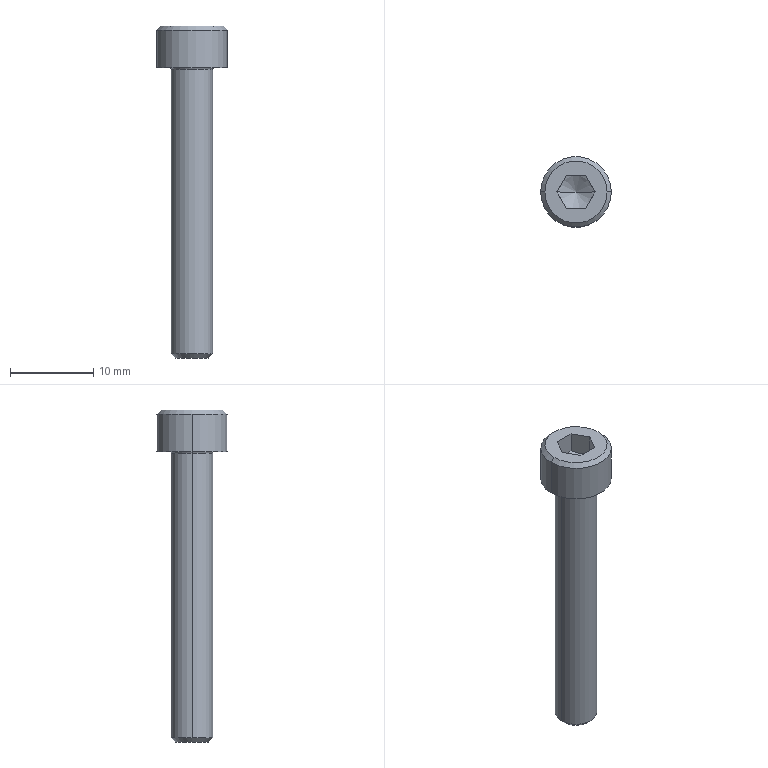Part | Creo | 1 solid | 23 faces | box 8.5 x 8.5 x 40 mm | volume 924.163 mm3 | plane 9 | cone 6 | cylinder 4 | torus 4 | commonest cylinder face diameters 5 x2 8.5 x2
STEP:
#1=CARTESIAN_POINT('',(0.,0.,0.));
#2=DIRECTION('',(0.,0.,1.));
#3=DIRECTION('',(1.,0.,0.));
#4=AXIS2_PLACEMENT_3D('',#1,#2,#3);
#5=CARTESIAN_POINT('',(-132.691,152.,16.));
#6=VERTEX_POINT('',#5);
#7=CARTESIAN_POINT('',(-133.845,154.,16.));
#8=VERTEX_POINT('',#7);
#9=CARTESIAN_POINT('',(-132.691,152.,16.));
#10=CARTESIAN_POINT('',(-132.753,152.109,15.964));
#11=CARTESIAN_POINT('',(-132.88,152.327,15.9));
#12=CARTESIAN_POINT('',(-133.073,152.663,15.836));
#13=CARTESIAN_POINT('',(-133.268,153.001,15.814));
#14=CARTESIAN_POINT('',(-133.464,153.339,15.836));
#15=CARTESIAN_POINT('',(-133.657,153.674,15.9));
#16=CARTESIAN_POINT('',(-133.783,153.892,15.964));
#17=CARTESIAN_POINT('',(-133.845,154.,16.));
#18=B_SPLINE_CURVE_WITH_KNOTS('',3,(#9,#10,#11,#12,#13,#14,#15,#16,#17),.UNSPECIFIED.,.F.,.F.,(4,1,1,1,1,1,4),(0.,0.1667,0.3333,0.5,0.6667,0.8333,1.),.UNSPECIFIED.);
#19=EDGE_CURVE('',#6,#8,#18,.T.);
#20=ORIENTED_EDGE('',*,*,#19,.F.);
#21=CARTESIAN_POINT('',(-135.,152.,14.667));
#22=VERTEX_POINT('',#21);
#23=CARTESIAN_POINT('',(-135.,152.,14.667));
#24=DIRECTION('',(0.866,0.,0.5));
#25=VECTOR('',#24,2.667);
#26=LINE('',#23,#25);
#27=EDGE_CURVE('',#22,#6,#26,.T.);
#28=ORIENTED_EDGE('',*,*,#27,.F.);
#29=CARTESIAN_POINT('',(-137.309,152.,16.));
#30=VERTEX_POINT('',#29);
#31=CARTESIAN_POINT('',(-135.,152.,14.667));
#32=DIRECTION('',(-0.866,0.,0.5));
#33=VECTOR('',#32,2.667);
#34=LINE('',#31,#33);
#35=EDGE_CURVE('',#22,#30,#34,.T.);
#36=ORIENTED_EDGE('',*,*,#35,.T.);
#37=CARTESIAN_POINT('',(-136.155,154.,16.));
#38=VERTEX_POINT('',#37);
#39=CARTESIAN_POINT('',(-136.155,154.,16.));
#40=CARTESIAN_POINT('',(-136.218,153.891,15.964));
#41=CARTESIAN_POINT('',(-136.344,153.673,15.9));
#42=CARTESIAN_POINT('',(-136.537,153.337,15.836));
#43=CARTESIAN_POINT('',(-136.733,152.999,15.814));
#44=CARTESIAN_POINT('',(-136.928,152.661,15.836));
#45=CARTESIAN_POINT('',(-137.121,152.326,15.9));
#46=CARTESIAN_POINT('',(-137.247,152.108,15.964));
#47=CARTESIAN_POINT('',(-137.309,152.,16.));
#48=B_SPLINE_CURVE_WITH_KNOTS('',3,(#39,#40,#41,#42,#43,#44,#45,#46,#47),.UNSPECIFIED.,.F.,.F.,(4,1,1,1,1,1,4),(0.,0.1667,0.3333,0.5,0.6667,0.8333,1.),.UNSPECIFIED.);
#49=EDGE_CURVE('',#38,#30,#48,.T.);
#50=ORIENTED_EDGE('',*,*,#49,.F.);
#51=CARTESIAN_POINT('',(-133.845,154.,16.));
#52=CARTESIAN_POINT('',(-133.919,154.,15.979));
#53=CARTESIAN_POINT('',(-134.064,154.,15.94));
#54=CARTESIAN_POINT('',(-134.273,154.,15.894));
#55=CARTESIAN_POINT('',(-134.479,154.,15.858));
#56=CARTESIAN_POINT('',(-134.685,154.,15.834));
#57=CARTESIAN_POINT('',(-134.895,154.,15.821));
#58=CARTESIAN_POINT('',(-135.105,154.,15.821));
#59=CARTESIAN_POINT('',(-135.315,154.,15.834));
#60=CARTESIAN_POINT('',(-135.521,154.,15.858));
#61=CARTESIAN_POINT('',(-135.727,154.,15.894));
#62=CARTESIAN_POINT('',(-135.936,154.,15.94));
#63=CARTESIAN_POINT('',(-136.081,154.,15.979));
#64=CARTESIAN_POINT('',(-136.155,154.,16.));
#65=B_SPLINE_CURVE_WITH_KNOTS('',3,(#51,#52,#53,#54,#55,#56,#57,#58,#59,#60,#61,#62,#63,#64),.UNSPECIFIED.,.F.,.F.,(4,1,1,1,1,1,1,1,1,1,1,4),(0.,0.09091,0.1818,0.2727,0.3636,0.4545,0.5455,0.6364,0.7273,0.8182,0.9091,1.),.UNSPECIFIED.);
#66=EDGE_CURVE('',#8,#38,#65,.T.);
#67=ORIENTED_EDGE('',*,*,#66,.F.);
#68=EDGE_LOOP('',(#20,#28,#36,#50,#67));
#69=FACE_OUTER_BOUND('',#68,.F.);
#70=CARTESIAN_POINT('',(-135.,152.,15.347));
#71=DIRECTION('',(0.,0.,1.));
#72=DIRECTION('',(1.,0.,0.));
#73=AXIS2_PLACEMENT_3D('',#70,#71,#72);
#74=CONICAL_SURFACE('',#73,1.178,60.);
#75=ADVANCED_FACE('',(#69),#74,.F.);
#76=CARTESIAN_POINT('',(-133.845,154.,18.5));
#77=VERTEX_POINT('',#76);
#78=CARTESIAN_POINT('',(-132.691,152.,18.5));
#79=VERTEX_POINT('',#78);
#80=CARTESIAN_POINT('',(-133.845,154.,18.5));
#81=DIRECTION('',(0.5,-0.866,0.));
#82=VECTOR('',#81,2.309);
#83=LINE('',#80,#82);
#84=EDGE_CURVE('',#77,#79,#83,.T.);
#85=ORIENTED_EDGE('',*,*,#84,.T.);
#86=CARTESIAN_POINT('',(-132.691,152.,18.5));
#87=DIRECTION('',(0.,0.,-1.));
#88=VECTOR('',#87,2.5);
#89=LINE('',#86,#88);
#90=EDGE_CURVE('',#79,#6,#89,.T.);
#91=ORIENTED_EDGE('',*,*,#90,.T.);
#92=ORIENTED_EDGE('',*,*,#19,.T.);
#93=CARTESIAN_POINT('',(-133.845,154.,18.5));
#94=DIRECTION('',(0.,0.,-1.));
#95=VECTOR('',#94,2.5);
#96=LINE('',#93,#95);
#97=EDGE_CURVE('',#77,#8,#96,.T.);
#98=ORIENTED_EDGE('',*,*,#97,.F.);
#99=EDGE_LOOP('',(#85,#91,#92,#98));
#100=FACE_OUTER_BOUND('',#99,.F.);
#101=CARTESIAN_POINT('',(-133.845,154.,16.));
#102=DIRECTION('',(-0.866,-0.5,0.));
#103=DIRECTION('',(0.5,-0.866,0.));
#104=AXIS2_PLACEMENT_3D('',#101,#102,#103);
#105=PLANE('',#104);
#106=ADVANCED_FACE('',(#100),#105,.T.);
#107=CARTESIAN_POINT('',(-131.25,152.,18.5));
#108=VERTEX_POINT('',#107);
#109=CARTESIAN_POINT('',(-138.75,152.,18.5));
#110=VERTEX_POINT('',#109);
#111=CARTESIAN_POINT('',(-135.,152.,18.5));
#112=DIRECTION('',(0.,0.,1.));
#113=DIRECTION('',(1.,0.,0.));
#114=AXIS2_PLACEMENT_3D('',#111,#112,#113);
#115=CIRCLE('',#114,3.75);
#116=EDGE_CURVE('',#108,#110,#115,.T.);
#117=ORIENTED_EDGE('',*,*,#116,.F.);
#118=CARTESIAN_POINT('',(-135.,152.,18.5));
#119=DIRECTION('',(0.,0.,1.));
#120=DIRECTION('',(-1.,0.,0.));
#121=AXIS2_PLACEMENT_3D('',#118,#119,#120);
#122=CIRCLE('',#121,3.75);
#123=EDGE_CURVE('',#110,#108,#122,.T.);
#124=ORIENTED_EDGE('',*,*,#123,.F.);
#125=EDGE_LOOP('',(#117,#124));
#126=FACE_OUTER_BOUND('',#125,.F.);
#127=CARTESIAN_POINT('',(-133.845,150.,18.5));
#128=VERTEX_POINT('',#127);
#129=CARTESIAN_POINT('',(-132.691,152.,18.5));
#130=DIRECTION('',(-0.5,-0.866,0.));
#131=VECTOR('',#130,2.309);
#132=LINE('',#129,#131);
#133=EDGE_CURVE('',#79,#128,#132,.T.);
#134=ORIENTED_EDGE('',*,*,#133,.F.);
#135=ORIENTED_EDGE('',*,*,#84,.F.);
#136=CARTESIAN_POINT('',(-136.155,154.,18.5));
#137=VERTEX_POINT('',#136);
#138=CARTESIAN_POINT('',(-133.845,154.,18.5));
#139=DIRECTION('',(-1.,0.,0.));
#140=VECTOR('',#139,2.309);
#141=LINE('',#138,#140);
#142=EDGE_CURVE('',#77,#137,#141,.T.);
#143=ORIENTED_EDGE('',*,*,#142,.T.);
#144=CARTESIAN_POINT('',(-137.309,152.,18.5));
#145=VERTEX_POINT('',#144);
#146=CARTESIAN_POINT('',(-137.309,152.,18.5));
#147=DIRECTION('',(0.5,0.866,0.));
#148=VECTOR('',#147,2.309);
#149=LINE('',#146,#148);
#150=EDGE_CURVE('',#145,#137,#149,.T.);
#151=ORIENTED_EDGE('',*,*,#150,.F.);
#152=CARTESIAN_POINT('',(-136.155,150.,18.5));
#153=VERTEX_POINT('',#152);
#154=CARTESIAN_POINT('',(-136.155,150.,18.5));
#155=DIRECTION('',(-0.5,0.866,0.));
#156=VECTOR('',#155,2.309);
#157=LINE('',#154,#156);
#158=EDGE_CURVE('',#153,#145,#157,.T.);
#159=ORIENTED_EDGE('',*,*,#158,.F.);
#160=CARTESIAN_POINT('',(-136.155,150.,18.5));
#161=DIRECTION('',(1.,0.,0.));
#162=VECTOR('',#161,2.309);
#163=LINE('',#160,#162);
#164=EDGE_CURVE('',#153,#128,#163,.T.);
#165=ORIENTED_EDGE('',*,*,#164,.T.);
#166=EDGE_LOOP('',(#134,#135,#143,#151,#159,#165));
#167=FACE_BOUND('',#166,.F.);
#168=CARTESIAN_POINT('',(-135.,152.,18.5));
#169=DIRECTION('',(0.,0.,1.));
#170=DIRECTION('',(1.,0.,0.));
#171=AXIS2_PLACEMENT_3D('',#168,#169,#170);
#172=PLANE('',#171);
#173=ADVANCED_FACE('',(#126,#167),#172,.T.);
#174=CARTESIAN_POINT('',(-130.75,152.,18.));
#175=VERTEX_POINT('',#174);
#176=CARTESIAN_POINT('',(-139.25,152.,18.));
#177=VERTEX_POINT('',#176);
#178=CARTESIAN_POINT('',(-135.,152.,18.));
#179=DIRECTION('',(0.,0.,1.));
#180=DIRECTION('',(1.,0.,0.));
#181=AXIS2_PLACEMENT_3D('',#178,#179,#180);
#182=CIRCLE('',#181,4.25);
#183=EDGE_CURVE('',#175,#177,#182,.T.);
#184=ORIENTED_EDGE('',*,*,#183,.F.);
#185=CARTESIAN_POINT('',(-131.25,152.,18.5));
#186=DIRECTION('',(0.7071,0.,-0.7071));
#187=VECTOR('',#186,0.7071);
#188=LINE('',#185,#187);
#189=EDGE_CURVE('',#108,#175,#188,.T.);
#190=ORIENTED_EDGE('',*,*,#189,.F.);
#191=ORIENTED_EDGE('',*,*,#116,.T.);
#192=CARTESIAN_POINT('',(-138.75,152.,18.5));
#193=DIRECTION('',(-0.7071,0.,-0.7071));
#194=VECTOR('',#193,0.7071);
#195=LINE('',#192,#194);
#196=EDGE_CURVE('',#110,#177,#195,.T.);
#197=ORIENTED_EDGE('',*,*,#196,.T.);
#198=EDGE_LOOP('',(#184,#190,#191,#197));
#199=FACE_OUTER_BOUND('',#198,.F.);
#200=CARTESIAN_POINT('',(-135.,152.,18.25));
#201=DIRECTION('',(0.,0.,-1.));
#202=DIRECTION('',(-1.,0.,0.));
#203=AXIS2_PLACEMENT_3D('',#200,#201,#202);
#204=CONICAL_SURFACE('',#203,4.,45.);
#205=ADVANCED_FACE('',(#199),#204,.T.);
#206=ORIENTED_EDGE('',*,*,#183,.T.);
#207=CARTESIAN_POINT('',(-139.25,152.,13.5));
#208=VERTEX_POINT('',#207);
#209=CARTESIAN_POINT('',(-139.25,152.,13.5));
#210=DIRECTION('',(0.,0.,1.));
#211=VECTOR('',#210,4.5);
#212=LINE('',#209,#211);
#213=EDGE_CURVE('',#208,#177,#212,.T.);
#214=ORIENTED_EDGE('',*,*,#213,.F.);
#215=CARTESIAN_POINT('',(-130.75,152.,13.5));
#216=VERTEX_POINT('',#215);
#217=CARTESIAN_POINT('',(-135.,152.,13.5));
#218=DIRECTION('',(0.,0.,-1.));
#219=DIRECTION('',(-1.,0.,0.));
#220=AXIS2_PLACEMENT_3D('',#217,#218,#219);
#221=CIRCLE('',#220,4.25);
#222=EDGE_CURVE('',#208,#216,#221,.T.);
#223=ORIENTED_EDGE('',*,*,#222,.T.);
#224=CARTESIAN_POINT('',(-130.75,152.,13.5));
#225=DIRECTION('',(0.,0.,1.));
#226=VECTOR('',#225,4.5);
#227=LINE('',#224,#226);
#228=EDGE_CURVE('',#216,#175,#227,.T.);
#229=ORIENTED_EDGE('',*,*,#228,.T.);
#230=EDGE_LOOP('',(#206,#214,#223,#229));
#231=FACE_OUTER_BOUND('',#230,.F.);
#232=CARTESIAN_POINT('',(-135.,152.,13.5));
#233=DIRECTION('',(0.,0.,1.));
#234=DIRECTION('',(1.,0.,0.));
#235=AXIS2_PLACEMENT_3D('',#232,#233,#234);
#236=CYLINDRICAL_SURFACE('',#235,4.25);
#237=ADVANCED_FACE('',(#231),#236,.T.);
#238=CARTESIAN_POINT('',(-135.,152.,18.));
#239=DIRECTION('',(0.,0.,1.));
#240=DIRECTION('',(-1.,0.,0.));
#241=AXIS2_PLACEMENT_3D('',#238,#239,#240);
#242=CIRCLE('',#241,4.25);
#243=EDGE_CURVE('',#177,#175,#242,.T.);
#244=ORIENTED_EDGE('',*,*,#243,.T.);
#245=ORIENTED_EDGE('',*,*,#228,.F.);
#246=CARTESIAN_POINT('',(-135.,152.,13.5));
#247=DIRECTION('',(0.,0.,-1.));
#248=DIRECTION('',(1.,0.,0.));
#249=AXIS2_PLACEMENT_3D('',#246,#247,#248);
#250=CIRCLE('',#249,4.25);
#251=EDGE_CURVE('',#216,#208,#250,.T.);
#252=ORIENTED_EDGE('',*,*,#251,.T.);
#253=ORIENTED_EDGE('',*,*,#213,.T.);
#254=EDGE_LOOP('',(#244,#245,#252,#253));
#255=FACE_OUTER_BOUND('',#254,.F.);
#256=CARTESIAN_POINT('',(-135.,152.,13.5));
#257=DIRECTION('',(0.,0.,1.));
#258=DIRECTION('',(1.,0.,0.));
#259=AXIS2_PLACEMENT_3D('',#256,#257,#258);
#260=CYLINDRICAL_SURFACE('',#259,4.25);
#261=ADVANCED_FACE('',(#255),#260,.T.);
#262=ORIENTED_EDGE('',*,*,#243,.F.);
#263=ORIENTED_EDGE('',*,*,#196,.F.);
#264=ORIENTED_EDGE('',*,*,#123,.T.);
#265=ORIENTED_EDGE('',*,*,#189,.T.);
#266=EDGE_LOOP('',(#262,#263,#264,#265));
#267=FACE_OUTER_BOUND('',#266,.F.);
#268=CARTESIAN_POINT('',(-135.,152.,18.25));
#269=DIRECTION('',(0.,0.,-1.));
#270=DIRECTION('',(-1.,0.,0.));
#271=AXIS2_PLACEMENT_3D('',#268,#269,#270);
#272=CONICAL_SURFACE('',#271,4.,45.);
#273=ADVANCED_FACE('',(#267),#272,.T.);
#274=ORIENTED_EDGE('',*,*,#251,.F.);
#275=ORIENTED_EDGE('',*,*,#222,.F.);
#276=EDGE_LOOP('',(#274,#275));
#277=FACE_OUTER_BOUND('',#276,.F.);
#278=CARTESIAN_POINT('',(-132.3,152.,13.5));
#279=VERTEX_POINT('',#278);
#280=CARTESIAN_POINT('',(-137.7,152.,13.5));
#281=VERTEX_POINT('',#280);
#282=CARTESIAN_POINT('',(-135.,152.,13.5));
#283=DIRECTION('',(0.,0.,1.));
#284=DIRECTION('',(1.,0.,0.));
#285=AXIS2_PLACEMENT_3D('',#282,#283,#284);
#286=CIRCLE('',#285,2.7);
#287=EDGE_CURVE('',#279,#281,#286,.T.);
#288=ORIENTED_EDGE('',*,*,#287,.F.);
#289=CARTESIAN_POINT('',(-135.,152.,13.5));
#290=DIRECTION('',(0.,0.,1.));
#291=DIRECTION('',(-1.,0.,0.));
#292=AXIS2_PLACEMENT_3D('',#289,#290,#291);
#293=CIRCLE('',#292,2.7);
#294=EDGE_CURVE('',#281,#279,#293,.T.);
#295=ORIENTED_EDGE('',*,*,#294,.F.);
#296=EDGE_LOOP('',(#288,#295));
#297=FACE_BOUND('',#296,.F.);
#298=CARTESIAN_POINT('',(-135.,152.,13.5));
#299=DIRECTION('',(0.,0.,1.));
#300=DIRECTION('',(1.,0.,0.));
#301=AXIS2_PLACEMENT_3D('',#298,#299,#300);
#302=PLANE('',#301);
#303=ADVANCED_FACE('',(#277,#297),#302,.F.);
#304=ORIENTED_EDGE('',*,*,#287,.T.);
#305=CARTESIAN_POINT('',(-137.559,152.,13.441));
#306=VERTEX_POINT('',#305);
#307=CARTESIAN_POINT('',(-137.7,152.,13.3));
#308=DIRECTION('',(0.,1.,0.));
#309=DIRECTION('',(0.,0.,1.));
#310=AXIS2_PLACEMENT_3D('',#307,#308,#309);
#311=CIRCLE('',#310,0.2);
#312=EDGE_CURVE('',#281,#306,#311,.T.);
#313=ORIENTED_EDGE('',*,*,#312,.T.);
#314=CARTESIAN_POINT('',(-132.441,152.,13.441));
#315=VERTEX_POINT('',#314);
#316=CARTESIAN_POINT('',(-135.,152.,13.441));
#317=DIRECTION('',(0.,0.,1.));
#318=DIRECTION('',(1.,0.,0.));
#319=AXIS2_PLACEMENT_3D('',#316,#317,#318);
#320=CIRCLE('',#319,2.559);
#321=EDGE_CURVE('',#315,#306,#320,.T.);
#322=ORIENTED_EDGE('',*,*,#321,.F.);
#323=CARTESIAN_POINT('',(-132.3,152.,13.3));
#324=DIRECTION('',(0.,-1.,0.));
#325=DIRECTION('',(0.,0.,1.));
#326=AXIS2_PLACEMENT_3D('',#323,#324,#325);
#327=CIRCLE('',#326,0.2);
#328=EDGE_CURVE('',#279,#315,#327,.T.);
#329=ORIENTED_EDGE('',*,*,#328,.F.);
#330=EDGE_LOOP('',(#304,#313,#322,#329));
#331=FACE_OUTER_BOUND('',#330,.F.);
#332=CARTESIAN_POINT('',(-135.,152.,13.3));
#333=DIRECTION('',(0.,0.,1.));
#334=DIRECTION('',(1.,0.,0.));
#335=AXIS2_PLACEMENT_3D('',#332,#333,#334);
#336=TOROIDAL_SURFACE('',#335,2.7,0.2);
#337=ADVANCED_FACE('',(#331),#336,.F.);
#338=ORIENTED_EDGE('',*,*,#294,.T.);
#339=ORIENTED_EDGE('',*,*,#328,.T.);
#340=CARTESIAN_POINT('',(-135.,152.,13.441));
#341=DIRECTION('',(0.,0.,1.));
#342=DIRECTION('',(-1.,0.,0.));
#343=AXIS2_PLACEMENT_3D('',#340,#341,#342);
#344=CIRCLE('',#343,2.559);
#345=EDGE_CURVE('',#306,#315,#344,.T.);
#346=ORIENTED_EDGE('',*,*,#345,.F.);
#347=ORIENTED_EDGE('',*,*,#312,.F.);
#348=EDGE_LOOP('',(#338,#339,#346,#347));
#349=FACE_OUTER_BOUND('',#348,.F.);
#350=CARTESIAN_POINT('',(-135.,152.,13.3));
#351=DIRECTION('',(0.,0.,1.));
#352=DIRECTION('',(1.,0.,0.));
#353=AXIS2_PLACEMENT_3D('',#350,#351,#352);
#354=TOROIDAL_SURFACE('',#353,2.7,0.2);
#355=ADVANCED_FACE('',(#349),#354,.F.);
#356=CARTESIAN_POINT('',(-137.5,152.,13.3));
#357=VERTEX_POINT('',#356);
#358=CARTESIAN_POINT('',(-132.5,152.,13.3));
#359=VERTEX_POINT('',#358);
#360=CARTESIAN_POINT('',(-135.,152.,13.3));
#361=DIRECTION('',(0.,0.,1.));
#362=DIRECTION('',(-1.,0.,0.));
#363=AXIS2_PLACEMENT_3D('',#360,#361,#362);
#364=CIRCLE('',#363,2.5);
#365=EDGE_CURVE('',#357,#359,#364,.T.);
#366=ORIENTED_EDGE('',*,*,#365,.F.);
#367=CARTESIAN_POINT('',(-137.7,152.,13.3));
#368=DIRECTION('',(0.,1.,0.));
#369=DIRECTION('',(0.7071,0.,0.7071));
#370=AXIS2_PLACEMENT_3D('',#367,#368,#369);
#371=CIRCLE('',#370,0.2);
#372=EDGE_CURVE('',#306,#357,#371,.T.);
#373=ORIENTED_EDGE('',*,*,#372,.F.);
#374=ORIENTED_EDGE('',*,*,#345,.T.);
#375=CARTESIAN_POINT('',(-132.3,152.,13.3));
#376=DIRECTION('',(0.,-1.,0.));
#377=DIRECTION('',(-0.7071,0.,0.7071));
#378=AXIS2_PLACEMENT_3D('',#375,#376,#377);
#379=CIRCLE('',#378,0.2);
#380=EDGE_CURVE('',#315,#359,#379,.T.);
#381=ORIENTED_EDGE('',*,*,#380,.T.);
#382=EDGE_LOOP('',(#366,#373,#374,#381));
#383=FACE_OUTER_BOUND('',#382,.F.);
#384=CARTESIAN_POINT('',(-135.,152.,13.3));
#385=DIRECTION('',(0.,0.,1.));
#386=DIRECTION('',(1.,0.,0.));
#387=AXIS2_PLACEMENT_3D('',#384,#385,#386);
#388=TOROIDAL_SURFACE('',#387,2.7,0.2);
#389=ADVANCED_FACE('',(#383),#388,.F.);
#390=CARTESIAN_POINT('',(-132.5,152.,-21.));
#391=VERTEX_POINT('',#390);
#392=CARTESIAN_POINT('',(-137.5,152.,-21.));
#393=VERTEX_POINT('',#392);
#394=CARTESIAN_POINT('',(-135.,152.,-21.));
#395=DIRECTION('',(0.,0.,-1.));
#396=DIRECTION('',(1.,0.,0.));
#397=AXIS2_PLACEMENT_3D('',#394,#395,#396);
#398=CIRCLE('',#397,2.5);
#399=EDGE_CURVE('',#391,#393,#398,.T.);
#400=ORIENTED_EDGE('',*,*,#399,.T.);
#401=CARTESIAN_POINT('',(-137.5,152.,-21.));
#402=DIRECTION('',(0.,0.,1.));
#403=VECTOR('',#402,34.3);
#404=LINE('',#401,#403);
#405=EDGE_CURVE('',#393,#357,#404,.T.);
#406=ORIENTED_EDGE('',*,*,#405,.T.);
#407=ORIENTED_EDGE('',*,*,#365,.T.);
#408=CARTESIAN_POINT('',(-132.5,152.,-21.));
#409=DIRECTION('',(0.,0.,1.));
#410=VECTOR('',#409,34.3);
#411=LINE('',#408,#410);
#412=EDGE_CURVE('',#391,#359,#411,.T.);
#413=ORIENTED_EDGE('',*,*,#412,.F.);
#414=EDGE_LOOP('',(#400,#406,#407,#413));
#415=FACE_OUTER_BOUND('',#414,.F.);
#416=CARTESIAN_POINT('',(-135.,152.,-21.5));
#417=DIRECTION('',(0.,0.,1.));
#418=DIRECTION('',(1.,0.,0.));
#419=AXIS2_PLACEMENT_3D('',#416,#417,#418);
#420=CYLINDRICAL_SURFACE('',#419,2.5);
#421=ADVANCED_FACE('',(#415),#420,.T.);
#422=CARTESIAN_POINT('',(-133.,152.,-21.5));
#423=VERTEX_POINT('',#422);
#424=CARTESIAN_POINT('',(-137.,152.,-21.5));
#425=VERTEX_POINT('',#424);
#426=CARTESIAN_POINT('',(-135.,152.,-21.5));
#427=DIRECTION('',(0.,0.,-1.));
#428=DIRECTION('',(1.,0.,0.));
#429=AXIS2_PLACEMENT_3D('',#426,#427,#428);
#430=CIRCLE('',#429,2.);
#431=EDGE_CURVE('',#423,#425,#430,.T.);
#432=ORIENTED_EDGE('',*,*,#431,.T.);
#433=CARTESIAN_POINT('',(-137.,152.,-21.5));
#434=DIRECTION('',(-0.7071,0.,0.7071));
#435=VECTOR('',#434,0.7071);
#436=LINE('',#433,#435);
#437=EDGE_CURVE('',#425,#393,#436,.T.);
#438=ORIENTED_EDGE('',*,*,#437,.T.);
#439=ORIENTED_EDGE('',*,*,#399,.F.);
#440=CARTESIAN_POINT('',(-133.,152.,-21.5));
#441=DIRECTION('',(0.7071,0.,0.7071));
#442=VECTOR('',#441,0.7071);
#443=LINE('',#440,#442);
#444=EDGE_CURVE('',#423,#391,#443,.T.);
#445=ORIENTED_EDGE('',*,*,#444,.F.);
#446=EDGE_LOOP('',(#432,#438,#439,#445));
#447=FACE_OUTER_BOUND('',#446,.F.);
#448=CARTESIAN_POINT('',(-135.,152.,-21.25));
#449=DIRECTION('',(0.,0.,1.));
#450=DIRECTION('',(1.,0.,0.));
#451=AXIS2_PLACEMENT_3D('',#448,#449,#450);
#452=CONICAL_SURFACE('',#451,2.25,45.);
#453=ADVANCED_FACE('',(#447),#452,.T.);
#454=ORIENTED_EDGE('',*,*,#431,.F.);
#455=CARTESIAN_POINT('',(-135.,152.,-21.5));
#456=DIRECTION('',(0.,0.,-1.));
#457=DIRECTION('',(-1.,0.,0.));
#458=AXIS2_PLACEMENT_3D('',#455,#456,#457);
#459=CIRCLE('',#458,2.);
#460=EDGE_CURVE('',#425,#423,#459,.T.);
#461=ORIENTED_EDGE('',*,*,#460,.F.);
#462=EDGE_LOOP('',(#454,#461));
#463=FACE_OUTER_BOUND('',#462,.F.);
#464=CARTESIAN_POINT('',(-135.,152.,-21.5));
#465=DIRECTION('',(0.,0.,1.));
#466=DIRECTION('',(1.,0.,0.));
#467=AXIS2_PLACEMENT_3D('',#464,#465,#466);
#468=PLANE('',#467);
#469=ADVANCED_FACE('',(#463),#468,.F.);
#470=ORIENTED_EDGE('',*,*,#460,.T.);
#471=ORIENTED_EDGE('',*,*,#444,.T.);
#472=CARTESIAN_POINT('',(-135.,152.,-21.));
#473=DIRECTION('',(0.,0.,-1.));
#474=DIRECTION('',(-1.,0.,0.));
#475=AXIS2_PLACEMENT_3D('',#472,#473,#474);
#476=CIRCLE('',#475,2.5);
#477=EDGE_CURVE('',#393,#391,#476,.T.);
#478=ORIENTED_EDGE('',*,*,#477,.F.);
#479=ORIENTED_EDGE('',*,*,#437,.F.);
#480=EDGE_LOOP('',(#470,#471,#478,#479));
#481=FACE_OUTER_BOUND('',#480,.F.);
#482=CARTESIAN_POINT('',(-135.,152.,-21.25));
#483=DIRECTION('',(0.,0.,1.));
#484=DIRECTION('',(1.,0.,0.));
#485=AXIS2_PLACEMENT_3D('',#482,#483,#484);
#486=CONICAL_SURFACE('',#485,2.25,45.);
#487=ADVANCED_FACE('',(#481),#486,.T.);
#488=ORIENTED_EDGE('',*,*,#477,.T.);
#489=ORIENTED_EDGE('',*,*,#412,.T.);
#490=CARTESIAN_POINT('',(-135.,152.,13.3));
#491=DIRECTION('',(0.,0.,1.));
#492=DIRECTION('',(1.,0.,0.));
#493=AXIS2_PLACEMENT_3D('',#490,#491,#492);
#494=CIRCLE('',#493,2.5);
#495=EDGE_CURVE('',#359,#357,#494,.T.);
#496=ORIENTED_EDGE('',*,*,#495,.T.);
#497=ORIENTED_EDGE('',*,*,#405,.F.);
#498=EDGE_LOOP('',(#488,#489,#496,#497));
#499=FACE_OUTER_BOUND('',#498,.F.);
#500=CARTESIAN_POINT('',(-135.,152.,-21.5));
#501=DIRECTION('',(0.,0.,1.));
#502=DIRECTION('',(1.,0.,0.));
#503=AXIS2_PLACEMENT_3D('',#500,#501,#502);
#504=CYLINDRICAL_SURFACE('',#503,2.5);
#505=ADVANCED_FACE('',(#499),#504,.T.);
#506=ORIENTED_EDGE('',*,*,#495,.F.);
#507=ORIENTED_EDGE('',*,*,#380,.F.);
#508=ORIENTED_EDGE('',*,*,#321,.T.);
#509=ORIENTED_EDGE('',*,*,#372,.T.);
#510=EDGE_LOOP('',(#506,#507,#508,#509));
#511=FACE_OUTER_BOUND('',#510,.F.);
#512=CARTESIAN_POINT('',(-135.,152.,13.3));
#513=DIRECTION('',(0.,0.,1.));
#514=DIRECTION('',(1.,0.,0.));
#515=AXIS2_PLACEMENT_3D('',#512,#513,#514);
#516=TOROIDAL_SURFACE('',#515,2.7,0.2);
#517=ADVANCED_FACE('',(#511),#516,.F.);
#518=ORIENTED_EDGE('',*,*,#133,.T.);
#519=CARTESIAN_POINT('',(-133.845,150.,16.));
#520=VERTEX_POINT('',#519);
#521=CARTESIAN_POINT('',(-133.845,150.,18.5));
#522=DIRECTION('',(0.,0.,-1.));
#523=VECTOR('',#522,2.5);
#524=LINE('',#521,#523);
#525=EDGE_CURVE('',#128,#520,#524,.T.);
#526=ORIENTED_EDGE('',*,*,#525,.T.);
#527=CARTESIAN_POINT('',(-133.845,150.,16.));
#528=CARTESIAN_POINT('',(-133.782,150.109,15.964));
#529=CARTESIAN_POINT('',(-133.656,150.327,15.9));
#530=CARTESIAN_POINT('',(-133.463,150.663,15.836));
#531=CARTESIAN_POINT('',(-133.267,151.001,15.814));
#532=CARTESIAN_POINT('',(-133.072,151.339,15.836));
#533=CARTESIAN_POINT('',(-132.879,151.674,15.9));
#534=CARTESIAN_POINT('',(-132.753,151.892,15.964));
#535=CARTESIAN_POINT('',(-132.691,152.,16.));
#536=B_SPLINE_CURVE_WITH_KNOTS('',3,(#527,#528,#529,#530,#531,#532,#533,#534,#535),.UNSPECIFIED.,.F.,.F.,(4,1,1,1,1,1,4),(0.,0.1667,0.3333,0.5,0.6667,0.8333,1.),.UNSPECIFIED.);
#537=EDGE_CURVE('',#520,#6,#536,.T.);
#538=ORIENTED_EDGE('',*,*,#537,.T.);
#539=ORIENTED_EDGE('',*,*,#90,.F.);
#540=EDGE_LOOP('',(#518,#526,#538,#539));
#541=FACE_OUTER_BOUND('',#540,.F.);
#542=CARTESIAN_POINT('',(-132.691,152.,16.));
#543=DIRECTION('',(-0.866,0.5,0.));
#544=DIRECTION('',(-0.5,-0.866,0.));
#545=AXIS2_PLACEMENT_3D('',#542,#543,#544);
#546=PLANE('',#545);
#547=ADVANCED_FACE('',(#541),#546,.T.);
#548=ORIENTED_EDGE('',*,*,#164,.F.);
#549=CARTESIAN_POINT('',(-136.155,150.,16.));
#550=VERTEX_POINT('',#549);
#551=CARTESIAN_POINT('',(-136.155,150.,18.5));
#552=DIRECTION('',(0.,0.,-1.));
#553=VECTOR('',#552,2.5);
#554=LINE('',#551,#553);
#555=EDGE_CURVE('',#153,#550,#554,.T.);
#556=ORIENTED_EDGE('',*,*,#555,.T.);
#557=CARTESIAN_POINT('',(-136.155,150.,16.));
#558=CARTESIAN_POINT('',(-136.081,150.,15.979));
#559=CARTESIAN_POINT('',(-135.936,150.,15.94));
#560=CARTESIAN_POINT('',(-135.727,150.,15.894));
#561=CARTESIAN_POINT('',(-135.521,150.,15.858));
#562=CARTESIAN_POINT('',(-135.315,150.,15.834));
#563=CARTESIAN_POINT('',(-135.105,150.,15.821));
#564=CARTESIAN_POINT('',(-134.895,150.,15.821));
#565=CARTESIAN_POINT('',(-134.685,150.,15.834));
#566=CARTESIAN_POINT('',(-134.479,150.,15.858));
#567=CARTESIAN_POINT('',(-134.273,150.,15.894));
#568=CARTESIAN_POINT('',(-134.064,150.,15.94));
#569=CARTESIAN_POINT('',(-133.919,150.,15.979));
#570=CARTESIAN_POINT('',(-133.845,150.,16.));
#571=B_SPLINE_CURVE_WITH_KNOTS('',3,(#557,#558,#559,#560,#561,#562,#563,#564,#565,#566,#567,#568,#569,#570),.UNSPECIFIED.,.F.,.F.,(4,1,1,1,1,1,1,1,1,1,1,4),(0.,0.09091,0.1818,0.2727,0.3636,0.4545,0.5455,0.6364,0.7273,0.8182,0.9091,1.),.UNSPECIFIED.);
#572=EDGE_CURVE('',#550,#520,#571,.T.);
#573=ORIENTED_EDGE('',*,*,#572,.T.);
#574=ORIENTED_EDGE('',*,*,#525,.F.);
#575=EDGE_LOOP('',(#548,#556,#573,#574));
#576=FACE_OUTER_BOUND('',#575,.F.);
#577=CARTESIAN_POINT('',(-133.845,150.,16.));
#578=DIRECTION('',(0.,1.,0.));
#579=DIRECTION('',(0.,0.,1.));
#580=AXIS2_PLACEMENT_3D('',#577,#578,#579);
#581=PLANE('',#580);
#582=ADVANCED_FACE('',(#576),#581,.T.);
#583=ORIENTED_EDGE('',*,*,#158,.T.);
#584=CARTESIAN_POINT('',(-137.309,152.,18.5));
#585=DIRECTION('',(0.,0.,-1.));
#586=VECTOR('',#585,2.5);
#587=LINE('',#584,#586);
#588=EDGE_CURVE('',#145,#30,#587,.T.);
#589=ORIENTED_EDGE('',*,*,#588,.T.);
#590=CARTESIAN_POINT('',(-137.309,152.,16.));
#591=CARTESIAN_POINT('',(-137.247,151.892,15.964));
#592=CARTESIAN_POINT('',(-137.121,151.674,15.9));
#593=CARTESIAN_POINT('',(-136.928,151.339,15.836));
#594=CARTESIAN_POINT('',(-136.733,151.001,15.814));
#595=CARTESIAN_POINT('',(-136.537,150.663,15.836));
#596=CARTESIAN_POINT('',(-136.344,150.327,15.9));
#597=CARTESIAN_POINT('',(-136.218,150.109,15.964));
#598=CARTESIAN_POINT('',(-136.155,150.,16.));
#599=B_SPLINE_CURVE_WITH_KNOTS('',3,(#590,#591,#592,#593,#594,#595,#596,#597,#598),.UNSPECIFIED.,.F.,.F.,(4,1,1,1,1,1,4),(0.,0.1667,0.3333,0.5,0.6667,0.8333,1.),.UNSPECIFIED.);
#600=EDGE_CURVE('',#30,#550,#599,.T.);
#601=ORIENTED_EDGE('',*,*,#600,.T.);
#602=ORIENTED_EDGE('',*,*,#555,.F.);
#603=EDGE_LOOP('',(#583,#589,#601,#602));
#604=FACE_OUTER_BOUND('',#603,.F.);
#605=CARTESIAN_POINT('',(-136.155,150.,16.));
#606=DIRECTION('',(0.866,0.5,0.));
#607=DIRECTION('',(-0.5,0.866,0.));
#608=AXIS2_PLACEMENT_3D('',#605,#606,#607);
#609=PLANE('',#608);
#610=ADVANCED_FACE('',(#604),#609,.T.);
#611=ORIENTED_EDGE('',*,*,#150,.T.);
#612=CARTESIAN_POINT('',(-136.155,154.,18.5));
#613=DIRECTION('',(0.,0.,-1.));
#614=VECTOR('',#613,2.5);
#615=LINE('',#612,#614);
#616=EDGE_CURVE('',#137,#38,#615,.T.);
#617=ORIENTED_EDGE('',*,*,#616,.T.);
#618=ORIENTED_EDGE('',*,*,#49,.T.);
#619=ORIENTED_EDGE('',*,*,#588,.F.);
#620=EDGE_LOOP('',(#611,#617,#618,#619));
#621=FACE_OUTER_BOUND('',#620,.F.);
#622=CARTESIAN_POINT('',(-137.309,152.,16.));
#623=DIRECTION('',(0.866,-0.5,0.));
#624=DIRECTION('',(0.5,0.866,0.));
#625=AXIS2_PLACEMENT_3D('',#622,#623,#624);
#626=PLANE('',#625);
#627=ADVANCED_FACE('',(#621),#626,.T.);
#628=ORIENTED_EDGE('',*,*,#142,.F.);
#629=ORIENTED_EDGE('',*,*,#97,.T.);
#630=ORIENTED_EDGE('',*,*,#66,.T.);
#631=ORIENTED_EDGE('',*,*,#616,.F.);
#632=EDGE_LOOP('',(#628,#629,#630,#631));
#633=FACE_OUTER_BOUND('',#632,.F.);
#634=CARTESIAN_POINT('',(-136.155,154.,16.));
#635=DIRECTION('',(0.,-1.,0.));
#636=DIRECTION('',(0.,0.,-1.));
#637=AXIS2_PLACEMENT_3D('',#634,#635,#636);
#638=PLANE('',#637);
#639=ADVANCED_FACE('',(#633),#638,.T.);
#640=ORIENTED_EDGE('',*,*,#600,.F.);
#641=ORIENTED_EDGE('',*,*,#35,.F.);
#642=ORIENTED_EDGE('',*,*,#27,.T.);
#643=ORIENTED_EDGE('',*,*,#537,.F.);
#644=ORIENTED_EDGE('',*,*,#572,.F.);
#645=EDGE_LOOP('',(#640,#641,#642,#643,#644));
#646=FACE_OUTER_BOUND('',#645,.F.);
#647=CARTESIAN_POINT('',(-135.,152.,15.347));
#648=DIRECTION('',(0.,0.,1.));
#649=DIRECTION('',(1.,0.,0.));
#650=AXIS2_PLACEMENT_3D('',#647,#648,#649);
#651=CONICAL_SURFACE('',#650,1.178,60.);
#652=ADVANCED_FACE('',(#646),#651,.F.);
#653=CLOSED_SHELL('',(#75,#106,#173,#205,#237,#261,#273,#303,#337,#355,#389,#421,#453,#469,#487,#505,#517,#547,#582,#610,#627,#639,#652));
#654=MANIFOLD_SOLID_BREP('',#653);
#655=(LENGTH_UNIT()NAMED_UNIT(*)SI_UNIT(.MILLI.,.METRE.));
#656=UNCERTAINTY_MEASURE_WITH_UNIT(LENGTH_MEASURE(0.004177),#655,'','');
#657=(NAMED_UNIT(*)PLANE_ANGLE_UNIT()SI_UNIT($,.RADIAN.));
#658=PLANE_ANGLE_MEASURE_WITH_UNIT(PLANE_ANGLE_MEASURE(0.01745),#657);
#659=(CONVERSION_BASED_UNIT('DEGREE',#658)NAMED_UNIT(*)PLANE_ANGLE_UNIT());
#660=(NAMED_UNIT(*)SI_UNIT($,.STERADIAN.)SOLID_ANGLE_UNIT());
#661=(GEOMETRIC_REPRESENTATION_CONTEXT(3)GLOBAL_UNCERTAINTY_ASSIGNED_CONTEXT((#656))GLOBAL_UNIT_ASSIGNED_CONTEXT((#655,#659,#660))REPRESENTATION_CONTEXT('',''));
#662=ADVANCED_BREP_SHAPE_REPRESENTATION('',(#4,#654),#661);